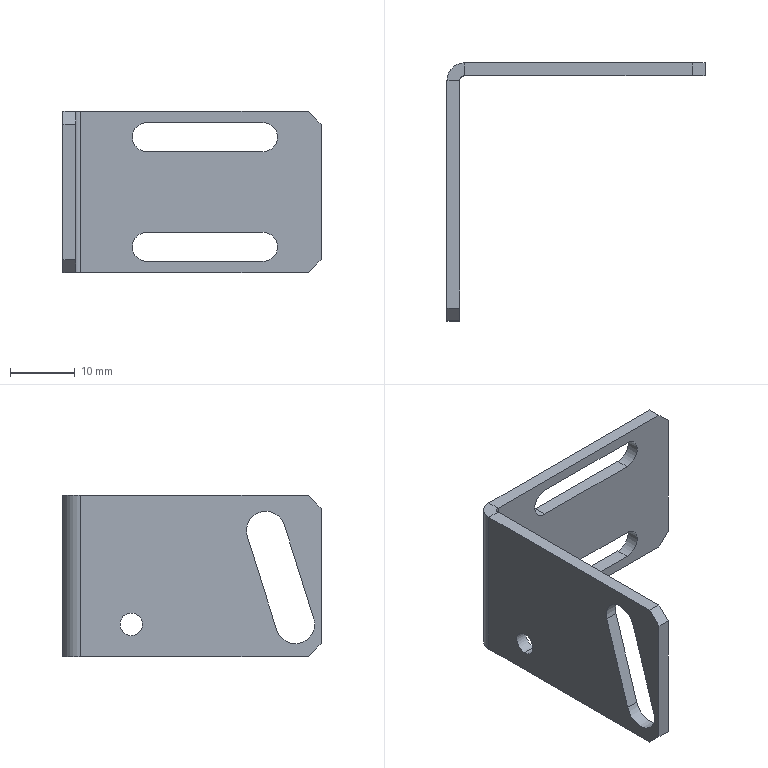Part | STEP file | CA-10-001Sensor Mount_Default | 1 solid | 33 faces | box 40 x 40 x 25 mm | volume 3201 mm3 | plane 22 | cylinder 11 | commonest cylinder face diameters 4.5 x4 6 x3 3.5 x2 1.473 x1 5.473 x1